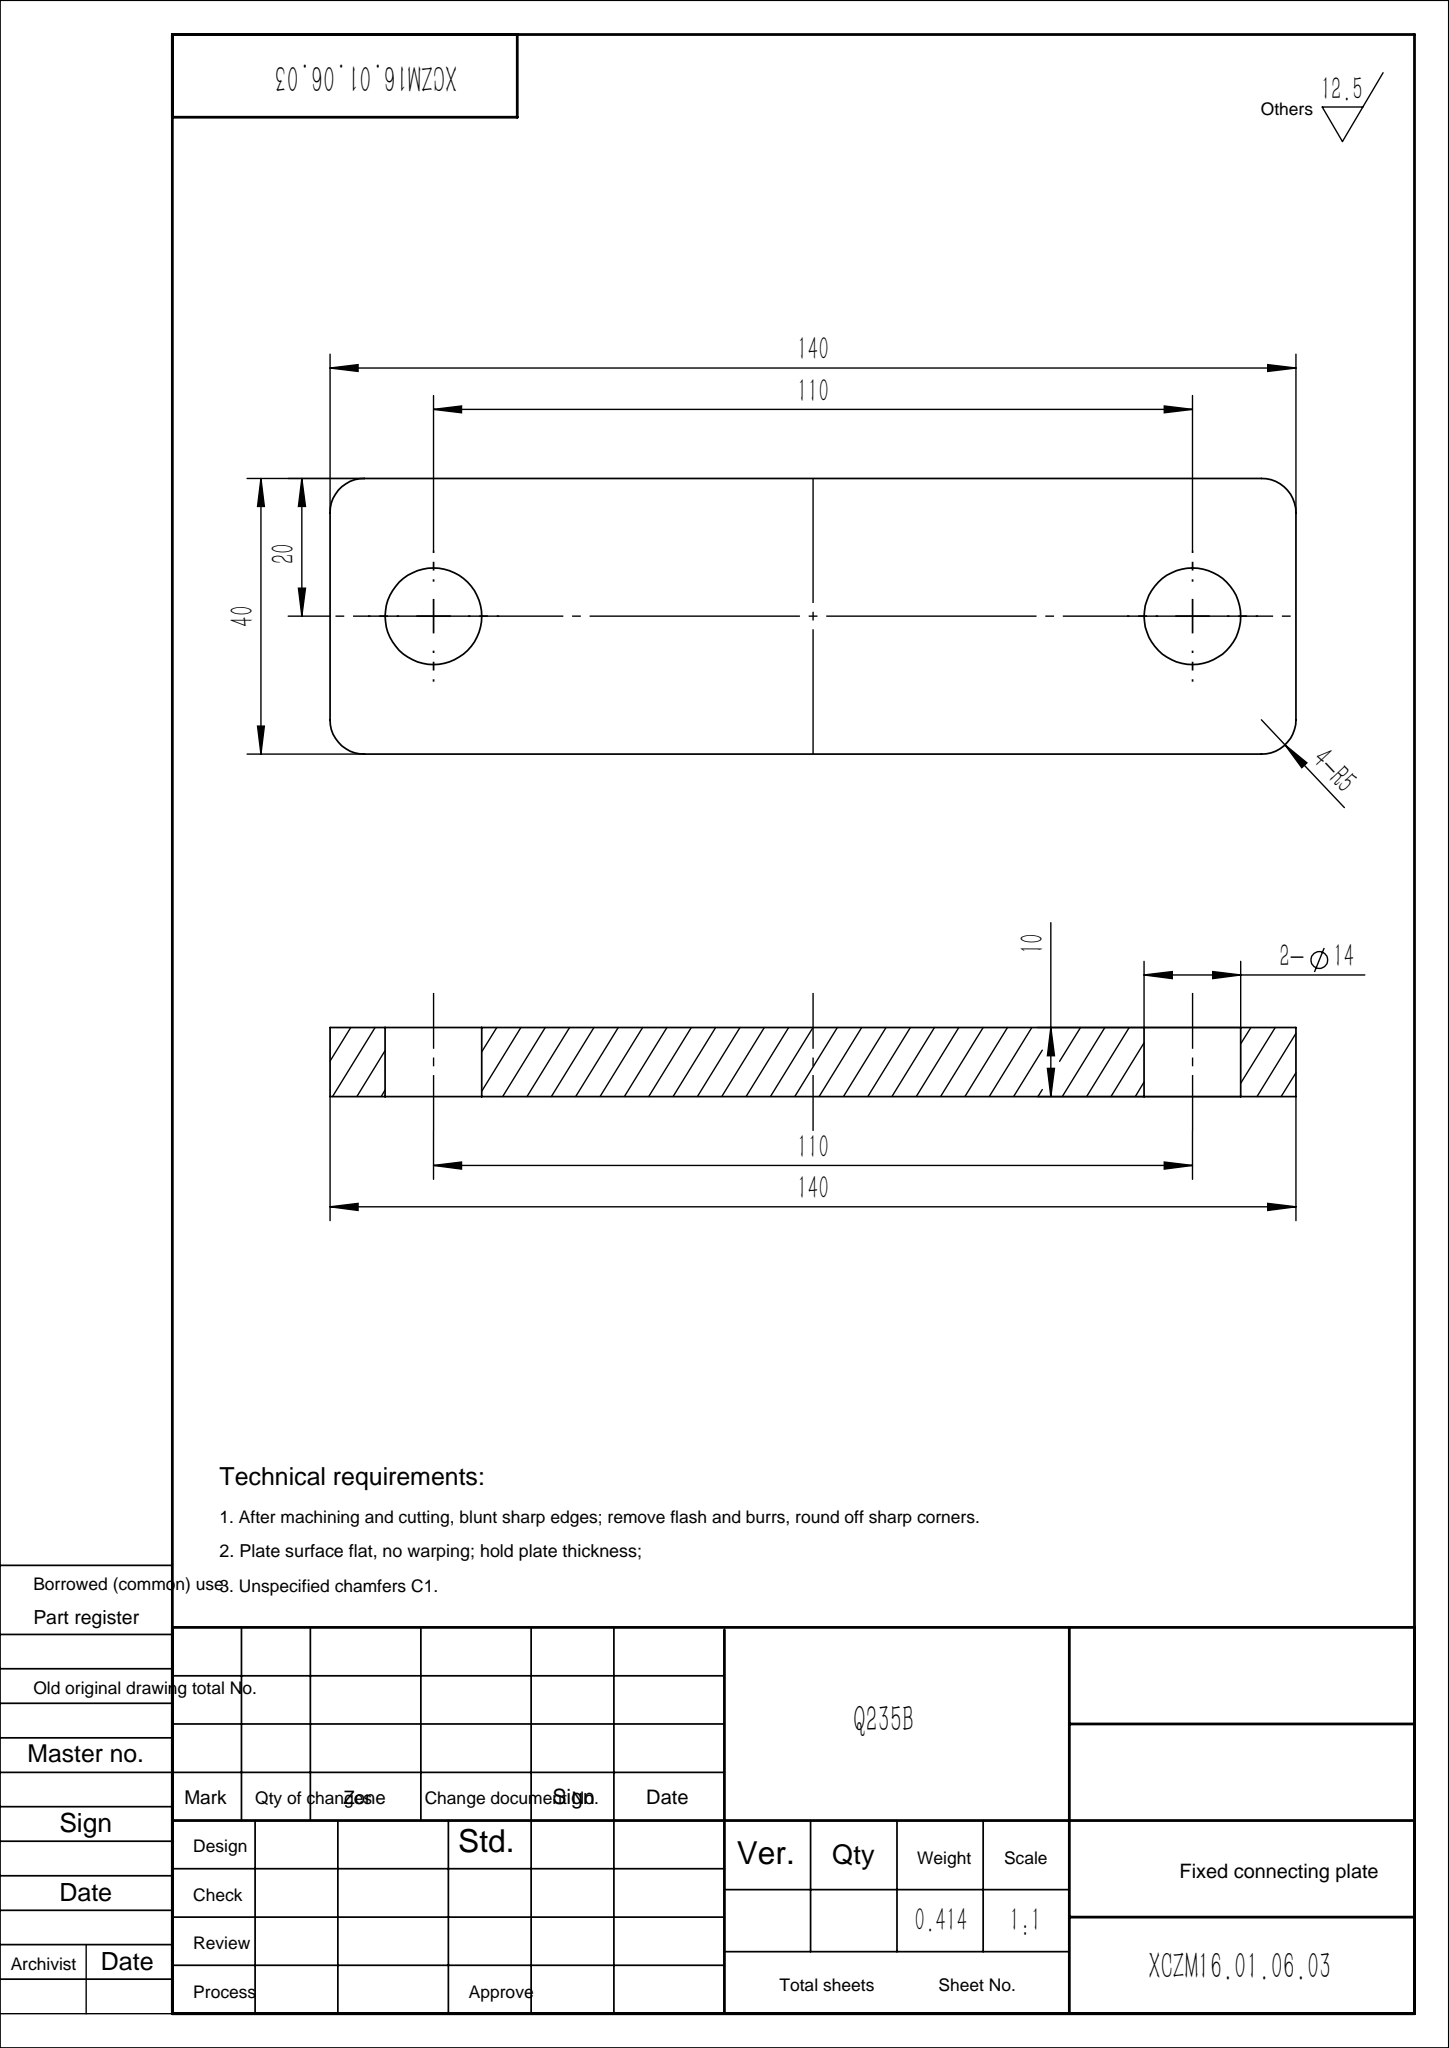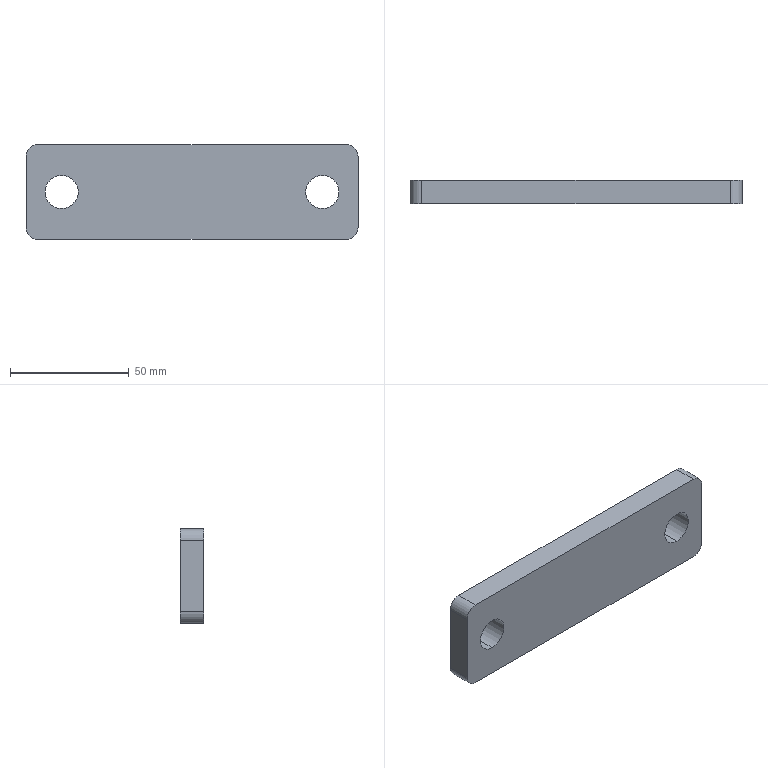Part | SolidWorks | features Extrusion 1 | 1 solid | 14 faces | box 140 x 10 x 40 mm | volume 52707 mm3 | cylinder 8 | plane 6 | commonest cylinder face diameters 10 x4 14 x4
STEP:
#1=CARTESIAN_POINT('',(55.,10.,-7.));
#2=VERTEX_POINT('',#1);
#3=CARTESIAN_POINT('',(55.,10.,7.));
#4=VERTEX_POINT('',#3);
#5=CARTESIAN_POINT('',(55.,10.,0.));
#6=DIRECTION('',(0.,1.,0.));
#7=DIRECTION('',(0.,0.,-1.));
#8=AXIS2_PLACEMENT_3D('',#5,#6,#7);
#9=CIRCLE('',#8,7.);
#10=EDGE_CURVE('',#2,#4,#9,.T.);
#11=ORIENTED_EDGE('',*,*,#10,.T.);
#12=CARTESIAN_POINT('',(55.,0.,7.));
#13=VERTEX_POINT('',#12);
#14=CARTESIAN_POINT('',(55.,10.,7.));
#15=DIRECTION('',(0.,-1.,0.));
#16=VECTOR('',#15,1000.);
#17=LINE('',#14,#16);
#18=EDGE_CURVE('',#4,#13,#17,.T.);
#19=ORIENTED_EDGE('',*,*,#18,.T.);
#20=CARTESIAN_POINT('',(55.,0.,-7.));
#21=VERTEX_POINT('',#20);
#22=CARTESIAN_POINT('',(55.,0.,0.));
#23=DIRECTION('',(0.,1.,0.));
#24=DIRECTION('',(0.,0.,-1.));
#25=AXIS2_PLACEMENT_3D('',#22,#23,#24);
#26=CIRCLE('',#25,7.);
#27=EDGE_CURVE('',#21,#13,#26,.T.);
#28=ORIENTED_EDGE('',*,*,#27,.F.);
#29=CARTESIAN_POINT('',(55.,10.,-7.));
#30=DIRECTION('',(0.,-1.,0.));
#31=VECTOR('',#30,1000.);
#32=LINE('',#29,#31);
#33=EDGE_CURVE('',#2,#21,#32,.T.);
#34=ORIENTED_EDGE('',*,*,#33,.F.);
#35=EDGE_LOOP('',(#11,#19,#28,#34));
#36=FACE_OUTER_BOUND('',#35,.T.);
#37=CARTESIAN_POINT('',(55.,10.,0.));
#38=DIRECTION('',(0.,-1.,0.));
#39=DIRECTION('',(0.,0.,-1.));
#40=AXIS2_PLACEMENT_3D('',#37,#38,#39);
#41=CYLINDRICAL_SURFACE('',#40,7.);
#42=ADVANCED_FACE('',(#36),#41,.F.);
#43=CARTESIAN_POINT('',(-55.,10.,-7.));
#44=VERTEX_POINT('',#43);
#45=CARTESIAN_POINT('',(-55.,10.,7.));
#46=VERTEX_POINT('',#45);
#47=CARTESIAN_POINT('',(-55.,10.,0.));
#48=DIRECTION('',(0.,1.,0.));
#49=DIRECTION('',(0.,0.,1.));
#50=AXIS2_PLACEMENT_3D('',#47,#48,#49);
#51=CIRCLE('',#50,7.);
#52=EDGE_CURVE('',#44,#46,#51,.T.);
#53=ORIENTED_EDGE('',*,*,#52,.T.);
#54=CARTESIAN_POINT('',(-55.,0.,7.));
#55=VERTEX_POINT('',#54);
#56=CARTESIAN_POINT('',(-55.,10.,7.));
#57=DIRECTION('',(0.,-1.,0.));
#58=VECTOR('',#57,1000.);
#59=LINE('',#56,#58);
#60=EDGE_CURVE('',#46,#55,#59,.T.);
#61=ORIENTED_EDGE('',*,*,#60,.T.);
#62=CARTESIAN_POINT('',(-55.,0.,-7.));
#63=VERTEX_POINT('',#62);
#64=CARTESIAN_POINT('',(-55.,0.,0.));
#65=DIRECTION('',(0.,1.,0.));
#66=DIRECTION('',(0.,0.,1.));
#67=AXIS2_PLACEMENT_3D('',#64,#65,#66);
#68=CIRCLE('',#67,7.);
#69=EDGE_CURVE('',#63,#55,#68,.T.);
#70=ORIENTED_EDGE('',*,*,#69,.F.);
#71=CARTESIAN_POINT('',(-55.,10.,-7.));
#72=DIRECTION('',(0.,-1.,0.));
#73=VECTOR('',#72,1000.);
#74=LINE('',#71,#73);
#75=EDGE_CURVE('',#44,#63,#74,.T.);
#76=ORIENTED_EDGE('',*,*,#75,.F.);
#77=EDGE_LOOP('',(#53,#61,#70,#76));
#78=FACE_OUTER_BOUND('',#77,.T.);
#79=CARTESIAN_POINT('',(-55.,10.,0.));
#80=DIRECTION('',(0.,-1.,0.));
#81=DIRECTION('',(0.,0.,-1.));
#82=AXIS2_PLACEMENT_3D('',#79,#80,#81);
#83=CYLINDRICAL_SURFACE('',#82,7.);
#84=ADVANCED_FACE('',(#78),#83,.F.);
#85=CARTESIAN_POINT('',(-70.,10.,15.));
#86=VERTEX_POINT('',#85);
#87=CARTESIAN_POINT('',(-65.,10.,20.));
#88=VERTEX_POINT('',#87);
#89=CARTESIAN_POINT('',(-65.,10.,15.));
#90=DIRECTION('',(0.,1.,0.));
#91=DIRECTION('',(0.,0.,-1.));
#92=AXIS2_PLACEMENT_3D('',#89,#90,#91);
#93=CIRCLE('',#92,5.);
#94=EDGE_CURVE('',#86,#88,#93,.T.);
#95=ORIENTED_EDGE('',*,*,#94,.T.);
#96=CARTESIAN_POINT('',(65.,10.,20.));
#97=VERTEX_POINT('',#96);
#98=CARTESIAN_POINT('',(65.,10.,20.));
#99=DIRECTION('',(1.,0.,0.));
#100=VECTOR('',#99,1000.);
#101=LINE('',#98,#100);
#102=EDGE_CURVE('',#88,#97,#101,.T.);
#103=ORIENTED_EDGE('',*,*,#102,.T.);
#104=CARTESIAN_POINT('',(70.,10.,15.));
#105=VERTEX_POINT('',#104);
#106=CARTESIAN_POINT('',(65.,10.,15.));
#107=DIRECTION('',(0.,1.,0.));
#108=DIRECTION('',(0.,0.,1.));
#109=AXIS2_PLACEMENT_3D('',#106,#107,#108);
#110=CIRCLE('',#109,5.);
#111=EDGE_CURVE('',#97,#105,#110,.T.);
#112=ORIENTED_EDGE('',*,*,#111,.T.);
#113=CARTESIAN_POINT('',(70.,10.,-15.));
#114=VERTEX_POINT('',#113);
#115=CARTESIAN_POINT('',(70.,10.,15.));
#116=DIRECTION('',(0.,0.,-1.));
#117=VECTOR('',#116,1000.);
#118=LINE('',#115,#117);
#119=EDGE_CURVE('',#105,#114,#118,.T.);
#120=ORIENTED_EDGE('',*,*,#119,.T.);
#121=CARTESIAN_POINT('',(65.,10.,-20.));
#122=VERTEX_POINT('',#121);
#123=CARTESIAN_POINT('',(65.,10.,-15.));
#124=DIRECTION('',(0.,1.,0.));
#125=DIRECTION('',(0.,0.,1.));
#126=AXIS2_PLACEMENT_3D('',#123,#124,#125);
#127=CIRCLE('',#126,5.);
#128=EDGE_CURVE('',#114,#122,#127,.T.);
#129=ORIENTED_EDGE('',*,*,#128,.T.);
#130=CARTESIAN_POINT('',(-65.,10.,-20.));
#131=VERTEX_POINT('',#130);
#132=CARTESIAN_POINT('',(65.,10.,-20.));
#133=DIRECTION('',(-1.,0.,0.));
#134=VECTOR('',#133,1000.);
#135=LINE('',#132,#134);
#136=EDGE_CURVE('',#122,#131,#135,.T.);
#137=ORIENTED_EDGE('',*,*,#136,.T.);
#138=CARTESIAN_POINT('',(-70.,10.,-15.));
#139=VERTEX_POINT('',#138);
#140=CARTESIAN_POINT('',(-65.,10.,-15.));
#141=DIRECTION('',(0.,1.,0.));
#142=DIRECTION('',(0.,0.,1.));
#143=AXIS2_PLACEMENT_3D('',#140,#141,#142);
#144=CIRCLE('',#143,5.);
#145=EDGE_CURVE('',#131,#139,#144,.T.);
#146=ORIENTED_EDGE('',*,*,#145,.T.);
#147=CARTESIAN_POINT('',(-70.,10.,15.));
#148=DIRECTION('',(0.,0.,1.));
#149=VECTOR('',#148,1000.);
#150=LINE('',#147,#149);
#151=EDGE_CURVE('',#139,#86,#150,.T.);
#152=ORIENTED_EDGE('',*,*,#151,.T.);
#153=EDGE_LOOP('',(#95,#103,#112,#120,#129,#137,#146,#152));
#154=FACE_OUTER_BOUND('',#153,.T.);
#155=ORIENTED_EDGE('',*,*,#52,.F.);
#156=CARTESIAN_POINT('',(-55.,10.,0.));
#157=DIRECTION('',(0.,1.,0.));
#158=DIRECTION('',(0.,0.,1.));
#159=AXIS2_PLACEMENT_3D('',#156,#157,#158);
#160=CIRCLE('',#159,7.);
#161=EDGE_CURVE('',#46,#44,#160,.T.);
#162=ORIENTED_EDGE('',*,*,#161,.F.);
#163=EDGE_LOOP('',(#155,#162));
#164=FACE_BOUND('',#163,.T.);
#165=ORIENTED_EDGE('',*,*,#10,.F.);
#166=CARTESIAN_POINT('',(55.,10.,0.));
#167=DIRECTION('',(0.,1.,0.));
#168=DIRECTION('',(0.,0.,-1.));
#169=AXIS2_PLACEMENT_3D('',#166,#167,#168);
#170=CIRCLE('',#169,7.);
#171=EDGE_CURVE('',#4,#2,#170,.T.);
#172=ORIENTED_EDGE('',*,*,#171,.F.);
#173=EDGE_LOOP('',(#165,#172));
#174=FACE_BOUND('',#173,.T.);
#175=CARTESIAN_POINT('',(-65.,10.,15.));
#176=DIRECTION('',(0.,-1.,0.));
#177=DIRECTION('',(0.,0.,-1.));
#178=AXIS2_PLACEMENT_3D('',#175,#176,#177);
#179=PLANE('',#178);
#180=ADVANCED_FACE('',(#154,#164,#174),#179,.F.);
#181=ORIENTED_EDGE('',*,*,#69,.T.);
#182=CARTESIAN_POINT('',(-55.,0.,0.));
#183=DIRECTION('',(0.,1.,0.));
#184=DIRECTION('',(0.,0.,1.));
#185=AXIS2_PLACEMENT_3D('',#182,#183,#184);
#186=CIRCLE('',#185,7.);
#187=EDGE_CURVE('',#55,#63,#186,.T.);
#188=ORIENTED_EDGE('',*,*,#187,.T.);
#189=EDGE_LOOP('',(#181,#188));
#190=FACE_BOUND('',#189,.T.);
#191=CARTESIAN_POINT('',(-70.,0.,15.));
#192=VERTEX_POINT('',#191);
#193=CARTESIAN_POINT('',(-65.,0.,20.));
#194=VERTEX_POINT('',#193);
#195=CARTESIAN_POINT('',(-65.,0.,15.));
#196=DIRECTION('',(0.,1.,0.));
#197=DIRECTION('',(0.,0.,-1.));
#198=AXIS2_PLACEMENT_3D('',#195,#196,#197);
#199=CIRCLE('',#198,5.);
#200=EDGE_CURVE('',#192,#194,#199,.T.);
#201=ORIENTED_EDGE('',*,*,#200,.F.);
#202=CARTESIAN_POINT('',(-70.,0.,-15.));
#203=VERTEX_POINT('',#202);
#204=CARTESIAN_POINT('',(-70.,0.,15.));
#205=DIRECTION('',(0.,0.,1.));
#206=VECTOR('',#205,1000.);
#207=LINE('',#204,#206);
#208=EDGE_CURVE('',#203,#192,#207,.T.);
#209=ORIENTED_EDGE('',*,*,#208,.F.);
#210=CARTESIAN_POINT('',(-65.,0.,-20.));
#211=VERTEX_POINT('',#210);
#212=CARTESIAN_POINT('',(-65.,0.,-15.));
#213=DIRECTION('',(0.,1.,0.));
#214=DIRECTION('',(0.,0.,1.));
#215=AXIS2_PLACEMENT_3D('',#212,#213,#214);
#216=CIRCLE('',#215,5.);
#217=EDGE_CURVE('',#211,#203,#216,.T.);
#218=ORIENTED_EDGE('',*,*,#217,.F.);
#219=CARTESIAN_POINT('',(65.,0.,-20.));
#220=VERTEX_POINT('',#219);
#221=CARTESIAN_POINT('',(65.,0.,-20.));
#222=DIRECTION('',(-1.,0.,0.));
#223=VECTOR('',#222,1000.);
#224=LINE('',#221,#223);
#225=EDGE_CURVE('',#220,#211,#224,.T.);
#226=ORIENTED_EDGE('',*,*,#225,.F.);
#227=CARTESIAN_POINT('',(70.,0.,-15.));
#228=VERTEX_POINT('',#227);
#229=CARTESIAN_POINT('',(65.,0.,-15.));
#230=DIRECTION('',(0.,1.,0.));
#231=DIRECTION('',(0.,0.,1.));
#232=AXIS2_PLACEMENT_3D('',#229,#230,#231);
#233=CIRCLE('',#232,5.);
#234=EDGE_CURVE('',#228,#220,#233,.T.);
#235=ORIENTED_EDGE('',*,*,#234,.F.);
#236=CARTESIAN_POINT('',(70.,0.,15.));
#237=VERTEX_POINT('',#236);
#238=CARTESIAN_POINT('',(70.,0.,15.));
#239=DIRECTION('',(0.,0.,-1.));
#240=VECTOR('',#239,1000.);
#241=LINE('',#238,#240);
#242=EDGE_CURVE('',#237,#228,#241,.T.);
#243=ORIENTED_EDGE('',*,*,#242,.F.);
#244=CARTESIAN_POINT('',(65.,0.,20.));
#245=VERTEX_POINT('',#244);
#246=CARTESIAN_POINT('',(65.,0.,15.));
#247=DIRECTION('',(0.,1.,0.));
#248=DIRECTION('',(0.,0.,1.));
#249=AXIS2_PLACEMENT_3D('',#246,#247,#248);
#250=CIRCLE('',#249,5.);
#251=EDGE_CURVE('',#245,#237,#250,.T.);
#252=ORIENTED_EDGE('',*,*,#251,.F.);
#253=CARTESIAN_POINT('',(65.,0.,20.));
#254=DIRECTION('',(1.,0.,0.));
#255=VECTOR('',#254,1000.);
#256=LINE('',#253,#255);
#257=EDGE_CURVE('',#194,#245,#256,.T.);
#258=ORIENTED_EDGE('',*,*,#257,.F.);
#259=EDGE_LOOP('',(#201,#209,#218,#226,#235,#243,#252,#258));
#260=FACE_OUTER_BOUND('',#259,.T.);
#261=ORIENTED_EDGE('',*,*,#27,.T.);
#262=CARTESIAN_POINT('',(55.,0.,0.));
#263=DIRECTION('',(0.,1.,0.));
#264=DIRECTION('',(0.,0.,-1.));
#265=AXIS2_PLACEMENT_3D('',#262,#263,#264);
#266=CIRCLE('',#265,7.);
#267=EDGE_CURVE('',#13,#21,#266,.T.);
#268=ORIENTED_EDGE('',*,*,#267,.T.);
#269=EDGE_LOOP('',(#261,#268));
#270=FACE_BOUND('',#269,.T.);
#271=CARTESIAN_POINT('',(-65.,0.,15.));
#272=DIRECTION('',(0.,-1.,0.));
#273=DIRECTION('',(0.,0.,-1.));
#274=AXIS2_PLACEMENT_3D('',#271,#272,#273);
#275=PLANE('',#274);
#276=ADVANCED_FACE('',(#190,#260,#270),#275,.T.);
#277=ORIENTED_EDGE('',*,*,#200,.T.);
#278=CARTESIAN_POINT('',(-65.,10.,20.));
#279=DIRECTION('',(0.,-1.,0.));
#280=VECTOR('',#279,1000.);
#281=LINE('',#278,#280);
#282=EDGE_CURVE('',#88,#194,#281,.T.);
#283=ORIENTED_EDGE('',*,*,#282,.F.);
#284=ORIENTED_EDGE('',*,*,#94,.F.);
#285=CARTESIAN_POINT('',(-70.,10.,15.));
#286=DIRECTION('',(0.,-1.,0.));
#287=VECTOR('',#286,1000.);
#288=LINE('',#285,#287);
#289=EDGE_CURVE('',#86,#192,#288,.T.);
#290=ORIENTED_EDGE('',*,*,#289,.T.);
#291=EDGE_LOOP('',(#277,#283,#284,#290));
#292=FACE_OUTER_BOUND('',#291,.T.);
#293=CARTESIAN_POINT('',(-65.,10.,15.));
#294=DIRECTION('',(0.,-1.,0.));
#295=DIRECTION('',(0.,0.,-1.));
#296=AXIS2_PLACEMENT_3D('',#293,#294,#295);
#297=CYLINDRICAL_SURFACE('',#296,5.);
#298=ADVANCED_FACE('',(#292),#297,.T.);
#299=ORIENTED_EDGE('',*,*,#257,.T.);
#300=CARTESIAN_POINT('',(65.,10.,20.));
#301=DIRECTION('',(0.,-1.,0.));
#302=VECTOR('',#301,1000.);
#303=LINE('',#300,#302);
#304=EDGE_CURVE('',#97,#245,#303,.T.);
#305=ORIENTED_EDGE('',*,*,#304,.F.);
#306=ORIENTED_EDGE('',*,*,#102,.F.);
#307=ORIENTED_EDGE('',*,*,#282,.T.);
#308=EDGE_LOOP('',(#299,#305,#306,#307));
#309=FACE_OUTER_BOUND('',#308,.T.);
#310=CARTESIAN_POINT('',(65.,10.,20.));
#311=DIRECTION('',(0.,0.,-1.));
#312=DIRECTION('',(-1.,0.,0.));
#313=AXIS2_PLACEMENT_3D('',#310,#311,#312);
#314=PLANE('',#313);
#315=ADVANCED_FACE('',(#309),#314,.F.);
#316=ORIENTED_EDGE('',*,*,#251,.T.);
#317=CARTESIAN_POINT('',(70.,10.,15.));
#318=DIRECTION('',(0.,-1.,0.));
#319=VECTOR('',#318,1000.);
#320=LINE('',#317,#319);
#321=EDGE_CURVE('',#105,#237,#320,.T.);
#322=ORIENTED_EDGE('',*,*,#321,.F.);
#323=ORIENTED_EDGE('',*,*,#111,.F.);
#324=ORIENTED_EDGE('',*,*,#304,.T.);
#325=EDGE_LOOP('',(#316,#322,#323,#324));
#326=FACE_OUTER_BOUND('',#325,.T.);
#327=CARTESIAN_POINT('',(65.,10.,15.));
#328=DIRECTION('',(0.,-1.,0.));
#329=DIRECTION('',(0.,0.,-1.));
#330=AXIS2_PLACEMENT_3D('',#327,#328,#329);
#331=CYLINDRICAL_SURFACE('',#330,5.);
#332=ADVANCED_FACE('',(#326),#331,.T.);
#333=ORIENTED_EDGE('',*,*,#242,.T.);
#334=CARTESIAN_POINT('',(70.,10.,-15.));
#335=DIRECTION('',(0.,-1.,0.));
#336=VECTOR('',#335,1000.);
#337=LINE('',#334,#336);
#338=EDGE_CURVE('',#114,#228,#337,.T.);
#339=ORIENTED_EDGE('',*,*,#338,.F.);
#340=ORIENTED_EDGE('',*,*,#119,.F.);
#341=ORIENTED_EDGE('',*,*,#321,.T.);
#342=EDGE_LOOP('',(#333,#339,#340,#341));
#343=FACE_OUTER_BOUND('',#342,.T.);
#344=CARTESIAN_POINT('',(70.,10.,15.));
#345=DIRECTION('',(-1.,0.,0.));
#346=DIRECTION('',(0.,0.,1.));
#347=AXIS2_PLACEMENT_3D('',#344,#345,#346);
#348=PLANE('',#347);
#349=ADVANCED_FACE('',(#343),#348,.F.);
#350=ORIENTED_EDGE('',*,*,#234,.T.);
#351=CARTESIAN_POINT('',(65.,10.,-20.));
#352=DIRECTION('',(0.,-1.,0.));
#353=VECTOR('',#352,1000.);
#354=LINE('',#351,#353);
#355=EDGE_CURVE('',#122,#220,#354,.T.);
#356=ORIENTED_EDGE('',*,*,#355,.F.);
#357=ORIENTED_EDGE('',*,*,#128,.F.);
#358=ORIENTED_EDGE('',*,*,#338,.T.);
#359=EDGE_LOOP('',(#350,#356,#357,#358));
#360=FACE_OUTER_BOUND('',#359,.T.);
#361=CARTESIAN_POINT('',(65.,10.,-15.));
#362=DIRECTION('',(0.,-1.,0.));
#363=DIRECTION('',(0.,0.,-1.));
#364=AXIS2_PLACEMENT_3D('',#361,#362,#363);
#365=CYLINDRICAL_SURFACE('',#364,5.);
#366=ADVANCED_FACE('',(#360),#365,.T.);
#367=ORIENTED_EDGE('',*,*,#225,.T.);
#368=CARTESIAN_POINT('',(-65.,10.,-20.));
#369=DIRECTION('',(0.,-1.,0.));
#370=VECTOR('',#369,1000.);
#371=LINE('',#368,#370);
#372=EDGE_CURVE('',#131,#211,#371,.T.);
#373=ORIENTED_EDGE('',*,*,#372,.F.);
#374=ORIENTED_EDGE('',*,*,#136,.F.);
#375=ORIENTED_EDGE('',*,*,#355,.T.);
#376=EDGE_LOOP('',(#367,#373,#374,#375));
#377=FACE_OUTER_BOUND('',#376,.T.);
#378=CARTESIAN_POINT('',(65.,10.,-20.));
#379=DIRECTION('',(0.,0.,1.));
#380=DIRECTION('',(1.,0.,0.));
#381=AXIS2_PLACEMENT_3D('',#378,#379,#380);
#382=PLANE('',#381);
#383=ADVANCED_FACE('',(#377),#382,.F.);
#384=ORIENTED_EDGE('',*,*,#217,.T.);
#385=CARTESIAN_POINT('',(-70.,10.,-15.));
#386=DIRECTION('',(0.,-1.,0.));
#387=VECTOR('',#386,1000.);
#388=LINE('',#385,#387);
#389=EDGE_CURVE('',#139,#203,#388,.T.);
#390=ORIENTED_EDGE('',*,*,#389,.F.);
#391=ORIENTED_EDGE('',*,*,#145,.F.);
#392=ORIENTED_EDGE('',*,*,#372,.T.);
#393=EDGE_LOOP('',(#384,#390,#391,#392));
#394=FACE_OUTER_BOUND('',#393,.T.);
#395=CARTESIAN_POINT('',(-65.,10.,-15.));
#396=DIRECTION('',(0.,-1.,0.));
#397=DIRECTION('',(0.,0.,-1.));
#398=AXIS2_PLACEMENT_3D('',#395,#396,#397);
#399=CYLINDRICAL_SURFACE('',#398,5.);
#400=ADVANCED_FACE('',(#394),#399,.T.);
#401=ORIENTED_EDGE('',*,*,#208,.T.);
#402=ORIENTED_EDGE('',*,*,#289,.F.);
#403=ORIENTED_EDGE('',*,*,#151,.F.);
#404=ORIENTED_EDGE('',*,*,#389,.T.);
#405=EDGE_LOOP('',(#401,#402,#403,#404));
#406=FACE_OUTER_BOUND('',#405,.T.);
#407=CARTESIAN_POINT('',(-70.,10.,15.));
#408=DIRECTION('',(1.,0.,0.));
#409=DIRECTION('',(0.,0.,-1.));
#410=AXIS2_PLACEMENT_3D('',#407,#408,#409);
#411=PLANE('',#410);
#412=ADVANCED_FACE('',(#406),#411,.F.);
#413=ORIENTED_EDGE('',*,*,#60,.F.);
#414=ORIENTED_EDGE('',*,*,#161,.T.);
#415=ORIENTED_EDGE('',*,*,#75,.T.);
#416=ORIENTED_EDGE('',*,*,#187,.F.);
#417=EDGE_LOOP('',(#413,#414,#415,#416));
#418=FACE_OUTER_BOUND('',#417,.T.);
#419=CARTESIAN_POINT('',(-55.,10.,0.));
#420=DIRECTION('',(0.,-1.,0.));
#421=DIRECTION('',(0.,0.,-1.));
#422=AXIS2_PLACEMENT_3D('',#419,#420,#421);
#423=CYLINDRICAL_SURFACE('',#422,7.);
#424=ADVANCED_FACE('',(#418),#423,.F.);
#425=ORIENTED_EDGE('',*,*,#18,.F.);
#426=ORIENTED_EDGE('',*,*,#171,.T.);
#427=ORIENTED_EDGE('',*,*,#33,.T.);
#428=ORIENTED_EDGE('',*,*,#267,.F.);
#429=EDGE_LOOP('',(#425,#426,#427,#428));
#430=FACE_OUTER_BOUND('',#429,.T.);
#431=CARTESIAN_POINT('',(55.,10.,0.));
#432=DIRECTION('',(0.,-1.,0.));
#433=DIRECTION('',(0.,0.,-1.));
#434=AXIS2_PLACEMENT_3D('',#431,#432,#433);
#435=CYLINDRICAL_SURFACE('',#434,7.);
#436=ADVANCED_FACE('',(#430),#435,.F.);
#437=CLOSED_SHELL('',(#42,#84,#180,#276,#298,#315,#332,#349,#366,#383,#400,#412,#424,#436));
#438=MANIFOLD_SOLID_BREP('',#437);
#439=CARTESIAN_POINT('',(0.,0.,0.));
#440=DIRECTION('',(0.,0.,1.));
#441=DIRECTION('',(1.,0.,0.));
#442=AXIS2_PLACEMENT_3D('',#439,#440,#441);
#443=(LENGTH_UNIT()NAMED_UNIT(*)SI_UNIT(.MILLI.,.METRE.));
#444=UNCERTAINTY_MEASURE_WITH_UNIT(LENGTH_MEASURE(0.00001),#443,'','');
#445=(NAMED_UNIT(*)PLANE_ANGLE_UNIT()SI_UNIT($,.RADIAN.));
#446=(NAMED_UNIT(*)SI_UNIT($,.STERADIAN.)SOLID_ANGLE_UNIT());
#447=(GEOMETRIC_REPRESENTATION_CONTEXT(3)GLOBAL_UNCERTAINTY_ASSIGNED_CONTEXT((#444))GLOBAL_UNIT_ASSIGNED_CONTEXT((#443,#445,#446))REPRESENTATION_CONTEXT('',''));
#448=ADVANCED_BREP_SHAPE_REPRESENTATION('',(#438,#442),#447);